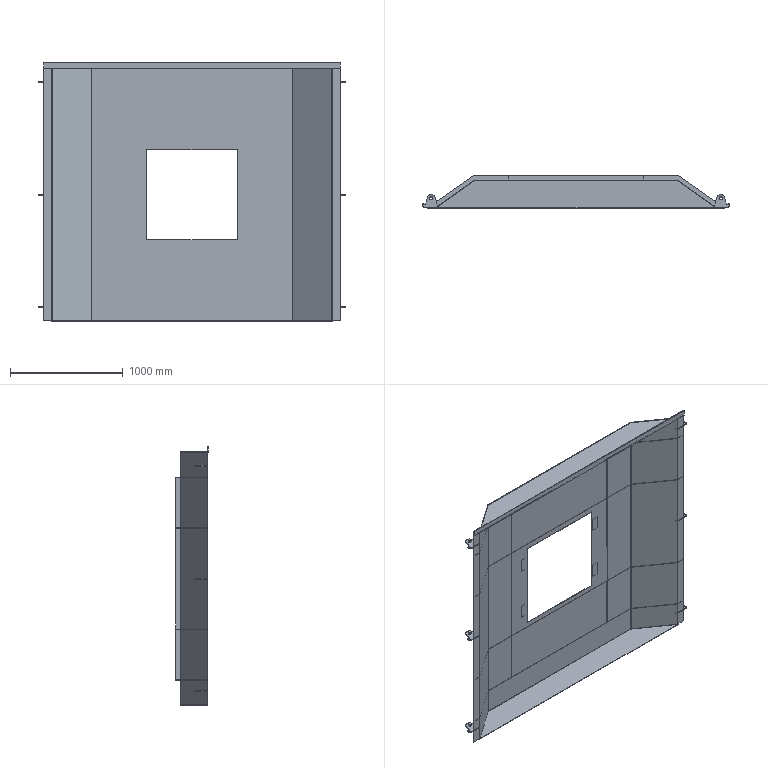Part | STEP file | Seal cover 2_Default<As machined> | 23 solids | 236 faces | box 2723 x 292.121 x 2296 mm | volume 30393848 mm3 | plane 198 | cylinder 38 | commonest cylinder face diameters 30 x18 16 x6 70 x6 6 x4 14 x4